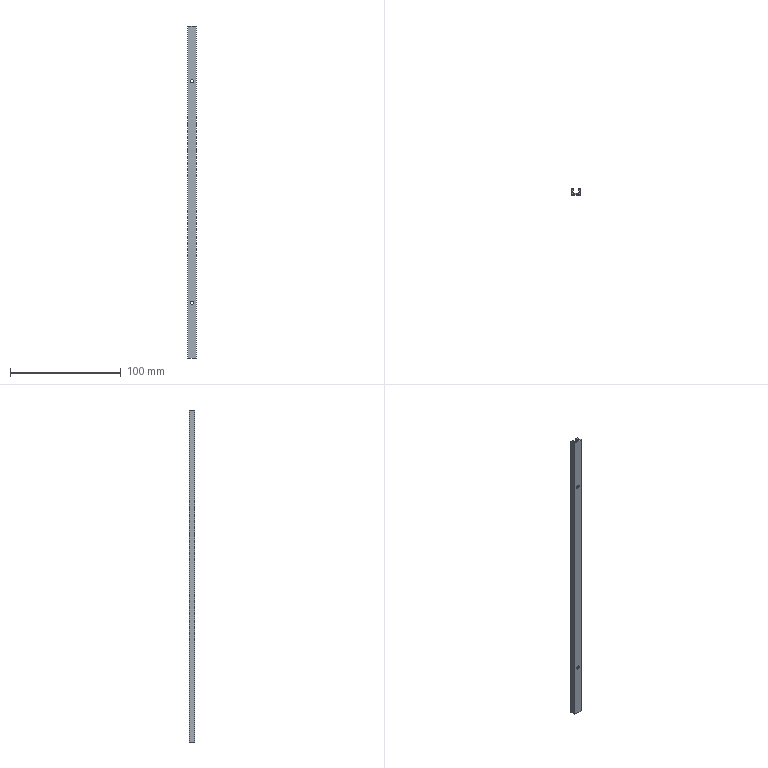Part | SolidWorks | features BaseBody 1 | 1 solid | 22 faces | box 8 x 5 x 300 mm | volume 5669 mm3 | plane 18 | cylinder 4 | commonest cylinder face diameters 3 x4
STEP:
#1=CARTESIAN_POINT('',(0.,0.9,226.5));
#2=VERTEX_POINT('',#1);
#3=CARTESIAN_POINT('',(0.,0.9,223.5));
#4=VERTEX_POINT('',#3);
#5=CARTESIAN_POINT('',(0.,0.9,225.));
#6=DIRECTION('',(0.,-1.,0.));
#7=DIRECTION('',(0.,0.,-1.));
#8=AXIS2_PLACEMENT_3D('',#5,#6,#7);
#9=CIRCLE('',#8,1.5);
#10=EDGE_CURVE('',#2,#4,#9,.T.);
#11=ORIENTED_EDGE('',*,*,#10,.F.);
#12=CARTESIAN_POINT('',(0.,0.,226.5));
#13=VERTEX_POINT('',#12);
#14=CARTESIAN_POINT('',(0.,4.,226.5));
#15=DIRECTION('',(0.,-1.,0.));
#16=VECTOR('',#15,1000.);
#17=LINE('',#14,#16);
#18=EDGE_CURVE('',#2,#13,#17,.T.);
#19=ORIENTED_EDGE('',*,*,#18,.T.);
#20=CARTESIAN_POINT('',(0.,0.,223.5));
#21=VERTEX_POINT('',#20);
#22=CARTESIAN_POINT('',(0.,0.,225.));
#23=DIRECTION('',(0.,1.,0.));
#24=DIRECTION('',(0.,0.,-1.));
#25=AXIS2_PLACEMENT_3D('',#22,#23,#24);
#26=CIRCLE('',#25,1.5);
#27=EDGE_CURVE('',#21,#13,#26,.T.);
#28=ORIENTED_EDGE('',*,*,#27,.F.);
#29=CARTESIAN_POINT('',(0.,4.,223.5));
#30=DIRECTION('',(0.,-1.,0.));
#31=VECTOR('',#30,1000.);
#32=LINE('',#29,#31);
#33=EDGE_CURVE('',#4,#21,#32,.T.);
#34=ORIENTED_EDGE('',*,*,#33,.F.);
#35=EDGE_LOOP('',(#11,#19,#28,#34));
#36=FACE_OUTER_BOUND('',#35,.T.);
#37=CARTESIAN_POINT('',(0.,4.,225.));
#38=DIRECTION('',(0.,-1.,0.));
#39=DIRECTION('',(0.,0.,-1.));
#40=AXIS2_PLACEMENT_3D('',#37,#38,#39);
#41=CYLINDRICAL_SURFACE('',#40,1.5);
#42=ADVANCED_FACE('',(#36),#41,.F.);
#43=CARTESIAN_POINT('',(0.,0.9,26.5));
#44=VERTEX_POINT('',#43);
#45=CARTESIAN_POINT('',(0.,0.9,23.5));
#46=VERTEX_POINT('',#45);
#47=CARTESIAN_POINT('',(0.,0.9,25.));
#48=DIRECTION('',(0.,-1.,0.));
#49=DIRECTION('',(0.,0.,-1.));
#50=AXIS2_PLACEMENT_3D('',#47,#48,#49);
#51=CIRCLE('',#50,1.5);
#52=EDGE_CURVE('',#44,#46,#51,.T.);
#53=ORIENTED_EDGE('',*,*,#52,.F.);
#54=CARTESIAN_POINT('',(0.,0.,26.5));
#55=VERTEX_POINT('',#54);
#56=CARTESIAN_POINT('',(0.,4.,26.5));
#57=DIRECTION('',(0.,-1.,0.));
#58=VECTOR('',#57,1000.);
#59=LINE('',#56,#58);
#60=EDGE_CURVE('',#44,#55,#59,.T.);
#61=ORIENTED_EDGE('',*,*,#60,.T.);
#62=CARTESIAN_POINT('',(0.,0.,23.5));
#63=VERTEX_POINT('',#62);
#64=CARTESIAN_POINT('',(0.,0.,25.));
#65=DIRECTION('',(0.,1.,0.));
#66=DIRECTION('',(0.,0.,-1.));
#67=AXIS2_PLACEMENT_3D('',#64,#65,#66);
#68=CIRCLE('',#67,1.5);
#69=EDGE_CURVE('',#63,#55,#68,.T.);
#70=ORIENTED_EDGE('',*,*,#69,.F.);
#71=CARTESIAN_POINT('',(0.,4.,23.5));
#72=DIRECTION('',(0.,-1.,0.));
#73=VECTOR('',#72,1000.);
#74=LINE('',#71,#73);
#75=EDGE_CURVE('',#46,#63,#74,.T.);
#76=ORIENTED_EDGE('',*,*,#75,.F.);
#77=EDGE_LOOP('',(#53,#61,#70,#76));
#78=FACE_OUTER_BOUND('',#77,.T.);
#79=CARTESIAN_POINT('',(0.,4.,25.));
#80=DIRECTION('',(0.,-1.,0.));
#81=DIRECTION('',(0.,0.,-1.));
#82=AXIS2_PLACEMENT_3D('',#79,#80,#81);
#83=CYLINDRICAL_SURFACE('',#82,1.5);
#84=ADVANCED_FACE('',(#78),#83,.F.);
#85=ORIENTED_EDGE('',*,*,#27,.T.);
#86=CARTESIAN_POINT('',(0.,0.,225.));
#87=DIRECTION('',(0.,1.,0.));
#88=DIRECTION('',(0.,0.,-1.));
#89=AXIS2_PLACEMENT_3D('',#86,#87,#88);
#90=CIRCLE('',#89,1.5);
#91=EDGE_CURVE('',#13,#21,#90,.T.);
#92=ORIENTED_EDGE('',*,*,#91,.T.);
#93=EDGE_LOOP('',(#85,#92));
#94=FACE_BOUND('',#93,.T.);
#95=ORIENTED_EDGE('',*,*,#69,.T.);
#96=CARTESIAN_POINT('',(0.,0.,25.));
#97=DIRECTION('',(0.,1.,0.));
#98=DIRECTION('',(0.,0.,-1.));
#99=AXIS2_PLACEMENT_3D('',#96,#97,#98);
#100=CIRCLE('',#99,1.5);
#101=EDGE_CURVE('',#55,#63,#100,.T.);
#102=ORIENTED_EDGE('',*,*,#101,.T.);
#103=EDGE_LOOP('',(#95,#102));
#104=FACE_BOUND('',#103,.T.);
#105=CARTESIAN_POINT('',(-4.,0.,-25.));
#106=VERTEX_POINT('',#105);
#107=CARTESIAN_POINT('',(4.,0.,-25.));
#108=VERTEX_POINT('',#107);
#109=CARTESIAN_POINT('',(-4.,0.,-25.));
#110=DIRECTION('',(1.,0.,0.));
#111=VECTOR('',#110,1000.);
#112=LINE('',#109,#111);
#113=EDGE_CURVE('',#106,#108,#112,.T.);
#114=ORIENTED_EDGE('',*,*,#113,.T.);
#115=CARTESIAN_POINT('',(4.,0.,275.));
#116=VERTEX_POINT('',#115);
#117=CARTESIAN_POINT('',(4.,0.,0.));
#118=DIRECTION('',(0.,0.,1.));
#119=VECTOR('',#118,1000.);
#120=LINE('',#117,#119);
#121=EDGE_CURVE('',#108,#116,#120,.T.);
#122=ORIENTED_EDGE('',*,*,#121,.T.);
#123=CARTESIAN_POINT('',(-4.,0.,275.));
#124=VERTEX_POINT('',#123);
#125=CARTESIAN_POINT('',(-4.,0.,275.));
#126=DIRECTION('',(-1.,0.,0.));
#127=VECTOR('',#126,1000.);
#128=LINE('',#125,#127);
#129=EDGE_CURVE('',#116,#124,#128,.T.);
#130=ORIENTED_EDGE('',*,*,#129,.T.);
#131=CARTESIAN_POINT('',(-4.,0.,0.));
#132=DIRECTION('',(0.,0.,-1.));
#133=VECTOR('',#132,1000.);
#134=LINE('',#131,#133);
#135=EDGE_CURVE('',#124,#106,#134,.T.);
#136=ORIENTED_EDGE('',*,*,#135,.T.);
#137=EDGE_LOOP('',(#114,#122,#130,#136));
#138=FACE_OUTER_BOUND('',#137,.T.);
#139=CARTESIAN_POINT('',(-4.,0.,0.));
#140=DIRECTION('',(0.,-1.,0.));
#141=DIRECTION('',(0.,0.,-1.));
#142=AXIS2_PLACEMENT_3D('',#139,#140,#141);
#143=PLANE('',#142);
#144=ADVANCED_FACE('',(#94,#104,#138),#143,.T.);
#145=ORIENTED_EDGE('',*,*,#18,.F.);
#146=CARTESIAN_POINT('',(0.,0.9,225.));
#147=DIRECTION('',(0.,-1.,0.));
#148=DIRECTION('',(0.,0.,-1.));
#149=AXIS2_PLACEMENT_3D('',#146,#147,#148);
#150=CIRCLE('',#149,1.5);
#151=EDGE_CURVE('',#4,#2,#150,.T.);
#152=ORIENTED_EDGE('',*,*,#151,.F.);
#153=ORIENTED_EDGE('',*,*,#33,.T.);
#154=ORIENTED_EDGE('',*,*,#91,.F.);
#155=EDGE_LOOP('',(#145,#152,#153,#154));
#156=FACE_OUTER_BOUND('',#155,.T.);
#157=CARTESIAN_POINT('',(0.,4.,225.));
#158=DIRECTION('',(0.,-1.,0.));
#159=DIRECTION('',(0.,0.,-1.));
#160=AXIS2_PLACEMENT_3D('',#157,#158,#159);
#161=CYLINDRICAL_SURFACE('',#160,1.5);
#162=ADVANCED_FACE('',(#156),#161,.F.);
#163=ORIENTED_EDGE('',*,*,#60,.F.);
#164=CARTESIAN_POINT('',(0.,0.9,25.));
#165=DIRECTION('',(0.,-1.,0.));
#166=DIRECTION('',(0.,0.,-1.));
#167=AXIS2_PLACEMENT_3D('',#164,#165,#166);
#168=CIRCLE('',#167,1.5);
#169=EDGE_CURVE('',#46,#44,#168,.T.);
#170=ORIENTED_EDGE('',*,*,#169,.F.);
#171=ORIENTED_EDGE('',*,*,#75,.T.);
#172=ORIENTED_EDGE('',*,*,#101,.F.);
#173=EDGE_LOOP('',(#163,#170,#171,#172));
#174=FACE_OUTER_BOUND('',#173,.T.);
#175=CARTESIAN_POINT('',(0.,4.,25.));
#176=DIRECTION('',(0.,-1.,0.));
#177=DIRECTION('',(0.,0.,-1.));
#178=AXIS2_PLACEMENT_3D('',#175,#176,#177);
#179=CYLINDRICAL_SURFACE('',#178,1.5);
#180=ADVANCED_FACE('',(#174),#179,.F.);
#181=CARTESIAN_POINT('',(4.,5.,275.));
#182=VERTEX_POINT('',#181);
#183=CARTESIAN_POINT('',(4.,0.,275.));
#184=DIRECTION('',(0.,-1.,0.));
#185=VECTOR('',#184,1000.);
#186=LINE('',#183,#185);
#187=EDGE_CURVE('',#182,#116,#186,.T.);
#188=ORIENTED_EDGE('',*,*,#187,.T.);
#189=ORIENTED_EDGE('',*,*,#121,.F.);
#190=CARTESIAN_POINT('',(4.,5.,-25.));
#191=VERTEX_POINT('',#190);
#192=CARTESIAN_POINT('',(4.,0.,-25.));
#193=DIRECTION('',(0.,1.,0.));
#194=VECTOR('',#193,1000.);
#195=LINE('',#192,#194);
#196=EDGE_CURVE('',#108,#191,#195,.T.);
#197=ORIENTED_EDGE('',*,*,#196,.T.);
#198=CARTESIAN_POINT('',(4.,5.,0.));
#199=DIRECTION('',(0.,0.,1.));
#200=VECTOR('',#199,1000.);
#201=LINE('',#198,#200);
#202=EDGE_CURVE('',#191,#182,#201,.T.);
#203=ORIENTED_EDGE('',*,*,#202,.T.);
#204=EDGE_LOOP('',(#188,#189,#197,#203));
#205=FACE_OUTER_BOUND('',#204,.T.);
#206=CARTESIAN_POINT('',(4.,0.,0.));
#207=DIRECTION('',(1.,0.,0.));
#208=DIRECTION('',(0.,0.,-1.));
#209=AXIS2_PLACEMENT_3D('',#206,#207,#208);
#210=PLANE('',#209);
#211=ADVANCED_FACE('',(#205),#210,.T.);
#212=ORIENTED_EDGE('',*,*,#113,.F.);
#213=CARTESIAN_POINT('',(-4.,5.,-25.));
#214=VERTEX_POINT('',#213);
#215=CARTESIAN_POINT('',(-4.,0.,-25.));
#216=DIRECTION('',(0.,-1.,0.));
#217=VECTOR('',#216,1000.);
#218=LINE('',#215,#217);
#219=EDGE_CURVE('',#214,#106,#218,.T.);
#220=ORIENTED_EDGE('',*,*,#219,.F.);
#221=CARTESIAN_POINT('',(-2.1,5.,-25.));
#222=VERTEX_POINT('',#221);
#223=CARTESIAN_POINT('',(0.,5.,-25.));
#224=DIRECTION('',(-1.,0.,0.));
#225=VECTOR('',#224,1000.);
#226=LINE('',#223,#225);
#227=EDGE_CURVE('',#222,#214,#226,.T.);
#228=ORIENTED_EDGE('',*,*,#227,.F.);
#229=CARTESIAN_POINT('',(-2.1,4.2,-25.));
#230=VERTEX_POINT('',#229);
#231=CARTESIAN_POINT('',(-2.1,4.2,-25.));
#232=DIRECTION('',(0.,1.,0.));
#233=VECTOR('',#232,1000.);
#234=LINE('',#231,#233);
#235=EDGE_CURVE('',#230,#222,#234,.T.);
#236=ORIENTED_EDGE('',*,*,#235,.F.);
#237=CARTESIAN_POINT('',(-2.9,4.2,-25.));
#238=VERTEX_POINT('',#237);
#239=CARTESIAN_POINT('',(-2.9,4.2,-25.));
#240=DIRECTION('',(1.,0.,0.));
#241=VECTOR('',#240,1000.);
#242=LINE('',#239,#241);
#243=EDGE_CURVE('',#238,#230,#242,.T.);
#244=ORIENTED_EDGE('',*,*,#243,.F.);
#245=CARTESIAN_POINT('',(-2.9,1.8,-25.));
#246=VERTEX_POINT('',#245);
#247=CARTESIAN_POINT('',(-2.9,0.,-25.));
#248=DIRECTION('',(0.,1.,0.));
#249=VECTOR('',#248,1000.);
#250=LINE('',#247,#249);
#251=EDGE_CURVE('',#246,#238,#250,.T.);
#252=ORIENTED_EDGE('',*,*,#251,.F.);
#253=CARTESIAN_POINT('',(-2.1,1.8,-25.));
#254=VERTEX_POINT('',#253);
#255=CARTESIAN_POINT('',(-2.1,1.8,-25.));
#256=DIRECTION('',(-1.,0.,0.));
#257=VECTOR('',#256,1000.);
#258=LINE('',#255,#257);
#259=EDGE_CURVE('',#254,#246,#258,.T.);
#260=ORIENTED_EDGE('',*,*,#259,.F.);
#261=CARTESIAN_POINT('',(-2.1,0.9,-25.));
#262=VERTEX_POINT('',#261);
#263=CARTESIAN_POINT('',(-2.1,0.9,-25.));
#264=DIRECTION('',(0.,1.,0.));
#265=VECTOR('',#264,1000.);
#266=LINE('',#263,#265);
#267=EDGE_CURVE('',#262,#254,#266,.T.);
#268=ORIENTED_EDGE('',*,*,#267,.F.);
#269=CARTESIAN_POINT('',(2.1,0.9,-25.));
#270=VERTEX_POINT('',#269);
#271=CARTESIAN_POINT('',(0.,0.9,-25.));
#272=DIRECTION('',(-1.,0.,0.));
#273=VECTOR('',#272,1000.);
#274=LINE('',#271,#273);
#275=EDGE_CURVE('',#270,#262,#274,.T.);
#276=ORIENTED_EDGE('',*,*,#275,.F.);
#277=CARTESIAN_POINT('',(2.1,1.8,-25.));
#278=VERTEX_POINT('',#277);
#279=CARTESIAN_POINT('',(2.1,1.8,-25.));
#280=DIRECTION('',(0.,-1.,0.));
#281=VECTOR('',#280,1000.);
#282=LINE('',#279,#281);
#283=EDGE_CURVE('',#278,#270,#282,.T.);
#284=ORIENTED_EDGE('',*,*,#283,.F.);
#285=CARTESIAN_POINT('',(2.9,1.8,-25.));
#286=VERTEX_POINT('',#285);
#287=CARTESIAN_POINT('',(2.9,1.8,-25.));
#288=DIRECTION('',(-1.,0.,0.));
#289=VECTOR('',#288,1000.);
#290=LINE('',#287,#289);
#291=EDGE_CURVE('',#286,#278,#290,.T.);
#292=ORIENTED_EDGE('',*,*,#291,.F.);
#293=CARTESIAN_POINT('',(2.9,4.2,-25.));
#294=VERTEX_POINT('',#293);
#295=CARTESIAN_POINT('',(2.9,0.,-25.));
#296=DIRECTION('',(0.,-1.,0.));
#297=VECTOR('',#296,1000.);
#298=LINE('',#295,#297);
#299=EDGE_CURVE('',#294,#286,#298,.T.);
#300=ORIENTED_EDGE('',*,*,#299,.F.);
#301=CARTESIAN_POINT('',(2.1,4.2,-25.));
#302=VERTEX_POINT('',#301);
#303=CARTESIAN_POINT('',(2.1,4.2,-25.));
#304=DIRECTION('',(1.,0.,0.));
#305=VECTOR('',#304,1000.);
#306=LINE('',#303,#305);
#307=EDGE_CURVE('',#302,#294,#306,.T.);
#308=ORIENTED_EDGE('',*,*,#307,.F.);
#309=CARTESIAN_POINT('',(2.1,5.,-25.));
#310=VERTEX_POINT('',#309);
#311=CARTESIAN_POINT('',(2.1,5.,-25.));
#312=DIRECTION('',(0.,-1.,0.));
#313=VECTOR('',#312,1000.);
#314=LINE('',#311,#313);
#315=EDGE_CURVE('',#310,#302,#314,.T.);
#316=ORIENTED_EDGE('',*,*,#315,.F.);
#317=CARTESIAN_POINT('',(0.,5.,-25.));
#318=DIRECTION('',(-1.,0.,0.));
#319=VECTOR('',#318,1000.);
#320=LINE('',#317,#319);
#321=EDGE_CURVE('',#191,#310,#320,.T.);
#322=ORIENTED_EDGE('',*,*,#321,.F.);
#323=ORIENTED_EDGE('',*,*,#196,.F.);
#324=EDGE_LOOP('',(#212,#220,#228,#236,#244,#252,#260,#268,#276,#284,#292,#300,#308,#316,#322,#323));
#325=FACE_OUTER_BOUND('',#324,.T.);
#326=CARTESIAN_POINT('',(0.,0.,-25.));
#327=DIRECTION('',(0.,0.,1.));
#328=DIRECTION('',(1.,0.,0.));
#329=AXIS2_PLACEMENT_3D('',#326,#327,#328);
#330=PLANE('',#329);
#331=ADVANCED_FACE('',(#325),#330,.F.);
#332=CARTESIAN_POINT('',(-4.,5.,275.));
#333=VERTEX_POINT('',#332);
#334=CARTESIAN_POINT('',(-4.,5.,275.));
#335=DIRECTION('',(0.,1.,0.));
#336=VECTOR('',#335,1000.);
#337=LINE('',#334,#336);
#338=EDGE_CURVE('',#124,#333,#337,.T.);
#339=ORIENTED_EDGE('',*,*,#338,.T.);
#340=CARTESIAN_POINT('',(-4.,5.,0.));
#341=DIRECTION('',(0.,0.,-1.));
#342=VECTOR('',#341,1000.);
#343=LINE('',#340,#342);
#344=EDGE_CURVE('',#333,#214,#343,.T.);
#345=ORIENTED_EDGE('',*,*,#344,.T.);
#346=ORIENTED_EDGE('',*,*,#219,.T.);
#347=ORIENTED_EDGE('',*,*,#135,.F.);
#348=EDGE_LOOP('',(#339,#345,#346,#347));
#349=FACE_OUTER_BOUND('',#348,.T.);
#350=CARTESIAN_POINT('',(-4.,5.,0.));
#351=DIRECTION('',(-1.,0.,0.));
#352=DIRECTION('',(0.,0.,1.));
#353=AXIS2_PLACEMENT_3D('',#350,#351,#352);
#354=PLANE('',#353);
#355=ADVANCED_FACE('',(#349),#354,.T.);
#356=CARTESIAN_POINT('',(2.1,1.8,275.));
#357=VERTEX_POINT('',#356);
#358=CARTESIAN_POINT('',(2.9,1.8,275.));
#359=VERTEX_POINT('',#358);
#360=CARTESIAN_POINT('',(2.9,1.8,275.));
#361=DIRECTION('',(1.,0.,0.));
#362=VECTOR('',#361,1000.);
#363=LINE('',#360,#362);
#364=EDGE_CURVE('',#357,#359,#363,.T.);
#365=ORIENTED_EDGE('',*,*,#364,.F.);
#366=CARTESIAN_POINT('',(2.1,0.9,275.));
#367=VERTEX_POINT('',#366);
#368=CARTESIAN_POINT('',(2.1,1.8,275.));
#369=DIRECTION('',(0.,1.,0.));
#370=VECTOR('',#369,1000.);
#371=LINE('',#368,#370);
#372=EDGE_CURVE('',#367,#357,#371,.T.);
#373=ORIENTED_EDGE('',*,*,#372,.F.);
#374=CARTESIAN_POINT('',(-2.1,0.9,275.));
#375=VERTEX_POINT('',#374);
#376=CARTESIAN_POINT('',(0.,0.9,275.));
#377=DIRECTION('',(-1.,0.,0.));
#378=VECTOR('',#377,1000.);
#379=LINE('',#376,#378);
#380=EDGE_CURVE('',#367,#375,#379,.T.);
#381=ORIENTED_EDGE('',*,*,#380,.T.);
#382=CARTESIAN_POINT('',(-2.1,1.8,275.));
#383=VERTEX_POINT('',#382);
#384=CARTESIAN_POINT('',(-2.1,0.9,275.));
#385=DIRECTION('',(0.,-1.,0.));
#386=VECTOR('',#385,1000.);
#387=LINE('',#384,#386);
#388=EDGE_CURVE('',#383,#375,#387,.T.);
#389=ORIENTED_EDGE('',*,*,#388,.F.);
#390=CARTESIAN_POINT('',(-2.9,1.8,275.));
#391=VERTEX_POINT('',#390);
#392=CARTESIAN_POINT('',(-2.1,1.8,275.));
#393=DIRECTION('',(1.,0.,0.));
#394=VECTOR('',#393,1000.);
#395=LINE('',#392,#394);
#396=EDGE_CURVE('',#391,#383,#395,.T.);
#397=ORIENTED_EDGE('',*,*,#396,.F.);
#398=CARTESIAN_POINT('',(-2.9,4.2,275.));
#399=VERTEX_POINT('',#398);
#400=CARTESIAN_POINT('',(-2.9,0.,275.));
#401=DIRECTION('',(0.,1.,0.));
#402=VECTOR('',#401,1000.);
#403=LINE('',#400,#402);
#404=EDGE_CURVE('',#391,#399,#403,.T.);
#405=ORIENTED_EDGE('',*,*,#404,.T.);
#406=CARTESIAN_POINT('',(-2.1,4.2,275.));
#407=VERTEX_POINT('',#406);
#408=CARTESIAN_POINT('',(-2.9,4.2,275.));
#409=DIRECTION('',(-1.,0.,0.));
#410=VECTOR('',#409,1000.);
#411=LINE('',#408,#410);
#412=EDGE_CURVE('',#407,#399,#411,.T.);
#413=ORIENTED_EDGE('',*,*,#412,.F.);
#414=CARTESIAN_POINT('',(-2.1,5.,275.));
#415=VERTEX_POINT('',#414);
#416=CARTESIAN_POINT('',(-2.1,4.2,275.));
#417=DIRECTION('',(0.,-1.,0.));
#418=VECTOR('',#417,1000.);
#419=LINE('',#416,#418);
#420=EDGE_CURVE('',#415,#407,#419,.T.);
#421=ORIENTED_EDGE('',*,*,#420,.F.);
#422=CARTESIAN_POINT('',(0.,5.,275.));
#423=DIRECTION('',(-1.,0.,0.));
#424=VECTOR('',#423,1000.);
#425=LINE('',#422,#424);
#426=EDGE_CURVE('',#415,#333,#425,.T.);
#427=ORIENTED_EDGE('',*,*,#426,.T.);
#428=ORIENTED_EDGE('',*,*,#338,.F.);
#429=ORIENTED_EDGE('',*,*,#129,.F.);
#430=ORIENTED_EDGE('',*,*,#187,.F.);
#431=CARTESIAN_POINT('',(2.1,5.,275.));
#432=VERTEX_POINT('',#431);
#433=CARTESIAN_POINT('',(0.,5.,275.));
#434=DIRECTION('',(-1.,0.,0.));
#435=VECTOR('',#434,1000.);
#436=LINE('',#433,#435);
#437=EDGE_CURVE('',#182,#432,#436,.T.);
#438=ORIENTED_EDGE('',*,*,#437,.T.);
#439=CARTESIAN_POINT('',(2.1,4.2,275.));
#440=VERTEX_POINT('',#439);
#441=CARTESIAN_POINT('',(2.1,5.,275.));
#442=DIRECTION('',(0.,1.,0.));
#443=VECTOR('',#442,1000.);
#444=LINE('',#441,#443);
#445=EDGE_CURVE('',#440,#432,#444,.T.);
#446=ORIENTED_EDGE('',*,*,#445,.F.);
#447=CARTESIAN_POINT('',(2.9,4.2,275.));
#448=VERTEX_POINT('',#447);
#449=CARTESIAN_POINT('',(2.1,4.2,275.));
#450=DIRECTION('',(-1.,0.,0.));
#451=VECTOR('',#450,1000.);
#452=LINE('',#449,#451);
#453=EDGE_CURVE('',#448,#440,#452,.T.);
#454=ORIENTED_EDGE('',*,*,#453,.F.);
#455=CARTESIAN_POINT('',(2.9,0.,275.));
#456=DIRECTION('',(0.,-1.,0.));
#457=VECTOR('',#456,1000.);
#458=LINE('',#455,#457);
#459=EDGE_CURVE('',#448,#359,#458,.T.);
#460=ORIENTED_EDGE('',*,*,#459,.T.);
#461=EDGE_LOOP('',(#365,#373,#381,#389,#397,#405,#413,#421,#427,#428,#429,#430,#438,#446,#454,#460));
#462=FACE_OUTER_BOUND('',#461,.T.);
#463=CARTESIAN_POINT('',(0.,0.,275.));
#464=DIRECTION('',(0.,0.,1.));
#465=DIRECTION('',(1.,0.,0.));
#466=AXIS2_PLACEMENT_3D('',#463,#464,#465);
#467=PLANE('',#466);
#468=ADVANCED_FACE('',(#462),#467,.T.);
#469=ORIENTED_EDGE('',*,*,#151,.T.);
#470=ORIENTED_EDGE('',*,*,#10,.T.);
#471=EDGE_LOOP('',(#469,#470));
#472=FACE_BOUND('',#471,.T.);
#473=ORIENTED_EDGE('',*,*,#169,.T.);
#474=ORIENTED_EDGE('',*,*,#52,.T.);
#475=EDGE_LOOP('',(#473,#474));
#476=FACE_BOUND('',#475,.T.);
#477=ORIENTED_EDGE('',*,*,#275,.T.);
#478=CARTESIAN_POINT('',(-2.1,0.9,0.));
#479=DIRECTION('',(0.,0.,1.));
#480=VECTOR('',#479,1000.);
#481=LINE('',#478,#480);
#482=EDGE_CURVE('',#262,#375,#481,.T.);
#483=ORIENTED_EDGE('',*,*,#482,.T.);
#484=ORIENTED_EDGE('',*,*,#380,.F.);
#485=CARTESIAN_POINT('',(2.1,0.9,0.));
#486=DIRECTION('',(0.,0.,-1.));
#487=VECTOR('',#486,1000.);
#488=LINE('',#485,#487);
#489=EDGE_CURVE('',#367,#270,#488,.T.);
#490=ORIENTED_EDGE('',*,*,#489,.T.);
#491=EDGE_LOOP('',(#477,#483,#484,#490));
#492=FACE_OUTER_BOUND('',#491,.T.);
#493=CARTESIAN_POINT('',(2.1,0.9,0.));
#494=DIRECTION('',(0.,1.,0.));
#495=DIRECTION('',(0.,0.,1.));
#496=AXIS2_PLACEMENT_3D('',#493,#494,#495);
#497=PLANE('',#496);
#498=ADVANCED_FACE('',(#472,#476,#492),#497,.T.);
#499=ORIENTED_EDGE('',*,*,#437,.F.);
#500=ORIENTED_EDGE('',*,*,#202,.F.);
#501=ORIENTED_EDGE('',*,*,#321,.T.);
#502=CARTESIAN_POINT('',(2.1,5.,0.));
#503=DIRECTION('',(0.,0.,1.));
#504=VECTOR('',#503,1000.);
#505=LINE('',#502,#504);
#506=EDGE_CURVE('',#310,#432,#505,.T.);
#507=ORIENTED_EDGE('',*,*,#506,.T.);
#508=EDGE_LOOP('',(#499,#500,#501,#507));
#509=FACE_OUTER_BOUND('',#508,.T.);
#510=CARTESIAN_POINT('',(4.,5.,0.));
#511=DIRECTION('',(0.,1.,0.));
#512=DIRECTION('',(0.,0.,1.));
#513=AXIS2_PLACEMENT_3D('',#510,#511,#512);
#514=PLANE('',#513);
#515=ADVANCED_FACE('',(#509),#514,.T.);
#516=ORIENTED_EDGE('',*,*,#426,.F.);
#517=CARTESIAN_POINT('',(-2.1,5.,0.));
#518=DIRECTION('',(0.,0.,-1.));
#519=VECTOR('',#518,1000.);
#520=LINE('',#517,#519);
#521=EDGE_CURVE('',#415,#222,#520,.T.);
#522=ORIENTED_EDGE('',*,*,#521,.T.);
#523=ORIENTED_EDGE('',*,*,#227,.T.);
#524=ORIENTED_EDGE('',*,*,#344,.F.);
#525=EDGE_LOOP('',(#516,#522,#523,#524));
#526=FACE_OUTER_BOUND('',#525,.T.);
#527=CARTESIAN_POINT('',(-2.1,5.,0.));
#528=DIRECTION('',(0.,1.,0.));
#529=DIRECTION('',(0.,0.,1.));
#530=AXIS2_PLACEMENT_3D('',#527,#528,#529);
#531=PLANE('',#530);
#532=ADVANCED_FACE('',(#526),#531,.T.);
#533=ORIENTED_EDGE('',*,*,#404,.F.);
#534=CARTESIAN_POINT('',(-2.9,1.8,0.));
#535=DIRECTION('',(0.,0.,-1.));
#536=VECTOR('',#535,1000.);
#537=LINE('',#534,#536);
#538=EDGE_CURVE('',#391,#246,#537,.T.);
#539=ORIENTED_EDGE('',*,*,#538,.T.);
#540=ORIENTED_EDGE('',*,*,#251,.T.);
#541=CARTESIAN_POINT('',(-2.9,4.2,0.));
#542=DIRECTION('',(0.,0.,1.));
#543=VECTOR('',#542,1000.);
#544=LINE('',#541,#543);
#545=EDGE_CURVE('',#238,#399,#544,.T.);
#546=ORIENTED_EDGE('',*,*,#545,.T.);
#547=EDGE_LOOP('',(#533,#539,#540,#546));
#548=FACE_OUTER_BOUND('',#547,.T.);
#549=CARTESIAN_POINT('',(-2.9,1.8,0.));
#550=DIRECTION('',(1.,0.,0.));
#551=DIRECTION('',(0.,0.,-1.));
#552=AXIS2_PLACEMENT_3D('',#549,#550,#551);
#553=PLANE('',#552);
#554=ADVANCED_FACE('',(#548),#553,.T.);
#555=ORIENTED_EDGE('',*,*,#459,.F.);
#556=CARTESIAN_POINT('',(2.9,4.2,0.));
#557=DIRECTION('',(0.,0.,-1.));
#558=VECTOR('',#557,1000.);
#559=LINE('',#556,#558);
#560=EDGE_CURVE('',#448,#294,#559,.T.);
#561=ORIENTED_EDGE('',*,*,#560,.T.);
#562=ORIENTED_EDGE('',*,*,#299,.T.);
#563=CARTESIAN_POINT('',(2.9,1.8,0.));
#564=DIRECTION('',(0.,0.,1.));
#565=VECTOR('',#564,1000.);
#566=LINE('',#563,#565);
#567=EDGE_CURVE('',#286,#359,#566,.T.);
#568=ORIENTED_EDGE('',*,*,#567,.T.);
#569=EDGE_LOOP('',(#555,#561,#562,#568));
#570=FACE_OUTER_BOUND('',#569,.T.);
#571=CARTESIAN_POINT('',(2.9,4.2,0.));
#572=DIRECTION('',(-1.,0.,0.));
#573=DIRECTION('',(0.,0.,1.));
#574=AXIS2_PLACEMENT_3D('',#571,#572,#573);
#575=PLANE('',#574);
#576=ADVANCED_FACE('',(#570),#575,.T.);
#577=ORIENTED_EDGE('',*,*,#388,.T.);
#578=ORIENTED_EDGE('',*,*,#482,.F.);
#579=ORIENTED_EDGE('',*,*,#267,.T.);
#580=CARTESIAN_POINT('',(-2.1,1.8,0.));
#581=DIRECTION('',(0.,0.,1.));
#582=VECTOR('',#581,1000.);
#583=LINE('',#580,#582);
#584=EDGE_CURVE('',#254,#383,#583,.T.);
#585=ORIENTED_EDGE('',*,*,#584,.T.);
#586=EDGE_LOOP('',(#577,#578,#579,#585));
#587=FACE_OUTER_BOUND('',#586,.T.);
#588=CARTESIAN_POINT('',(-2.1,0.9,0.));
#589=DIRECTION('',(1.,0.,0.));
#590=DIRECTION('',(0.,0.,-1.));
#591=AXIS2_PLACEMENT_3D('',#588,#589,#590);
#592=PLANE('',#591);
#593=ADVANCED_FACE('',(#587),#592,.T.);
#594=ORIENTED_EDGE('',*,*,#372,.T.);
#595=CARTESIAN_POINT('',(2.1,1.8,0.));
#596=DIRECTION('',(0.,0.,-1.));
#597=VECTOR('',#596,1000.);
#598=LINE('',#595,#597);
#599=EDGE_CURVE('',#357,#278,#598,.T.);
#600=ORIENTED_EDGE('',*,*,#599,.T.);
#601=ORIENTED_EDGE('',*,*,#283,.T.);
#602=ORIENTED_EDGE('',*,*,#489,.F.);
#603=EDGE_LOOP('',(#594,#600,#601,#602));
#604=FACE_OUTER_BOUND('',#603,.T.);
#605=CARTESIAN_POINT('',(2.1,1.8,0.));
#606=DIRECTION('',(-1.,0.,0.));
#607=DIRECTION('',(0.,0.,1.));
#608=AXIS2_PLACEMENT_3D('',#605,#606,#607);
#609=PLANE('',#608);
#610=ADVANCED_FACE('',(#604),#609,.T.);
#611=ORIENTED_EDGE('',*,*,#445,.T.);
#612=ORIENTED_EDGE('',*,*,#506,.F.);
#613=ORIENTED_EDGE('',*,*,#315,.T.);
#614=CARTESIAN_POINT('',(2.1,4.2,0.));
#615=DIRECTION('',(0.,0.,1.));
#616=VECTOR('',#615,1000.);
#617=LINE('',#614,#616);
#618=EDGE_CURVE('',#302,#440,#617,.T.);
#619=ORIENTED_EDGE('',*,*,#618,.T.);
#620=EDGE_LOOP('',(#611,#612,#613,#619));
#621=FACE_OUTER_BOUND('',#620,.T.);
#622=CARTESIAN_POINT('',(2.1,5.,0.));
#623=DIRECTION('',(-1.,0.,0.));
#624=DIRECTION('',(0.,0.,1.));
#625=AXIS2_PLACEMENT_3D('',#622,#623,#624);
#626=PLANE('',#625);
#627=ADVANCED_FACE('',(#621),#626,.T.);
#628=ORIENTED_EDGE('',*,*,#420,.T.);
#629=CARTESIAN_POINT('',(-2.1,4.2,0.));
#630=DIRECTION('',(0.,0.,-1.));
#631=VECTOR('',#630,1000.);
#632=LINE('',#629,#631);
#633=EDGE_CURVE('',#407,#230,#632,.T.);
#634=ORIENTED_EDGE('',*,*,#633,.T.);
#635=ORIENTED_EDGE('',*,*,#235,.T.);
#636=ORIENTED_EDGE('',*,*,#521,.F.);
#637=EDGE_LOOP('',(#628,#634,#635,#636));
#638=FACE_OUTER_BOUND('',#637,.T.);
#639=CARTESIAN_POINT('',(-2.1,4.2,0.));
#640=DIRECTION('',(1.,0.,0.));
#641=DIRECTION('',(0.,0.,-1.));
#642=AXIS2_PLACEMENT_3D('',#639,#640,#641);
#643=PLANE('',#642);
#644=ADVANCED_FACE('',(#638),#643,.T.);
#645=ORIENTED_EDGE('',*,*,#396,.T.);
#646=ORIENTED_EDGE('',*,*,#584,.F.);
#647=ORIENTED_EDGE('',*,*,#259,.T.);
#648=ORIENTED_EDGE('',*,*,#538,.F.);
#649=EDGE_LOOP('',(#645,#646,#647,#648));
#650=FACE_OUTER_BOUND('',#649,.T.);
#651=CARTESIAN_POINT('',(-2.1,1.8,0.));
#652=DIRECTION('',(0.,1.,0.));
#653=DIRECTION('',(0.,0.,1.));
#654=AXIS2_PLACEMENT_3D('',#651,#652,#653);
#655=PLANE('',#654);
#656=ADVANCED_FACE('',(#650),#655,.T.);
#657=ORIENTED_EDGE('',*,*,#412,.T.);
#658=ORIENTED_EDGE('',*,*,#545,.F.);
#659=ORIENTED_EDGE('',*,*,#243,.T.);
#660=ORIENTED_EDGE('',*,*,#633,.F.);
#661=EDGE_LOOP('',(#657,#658,#659,#660));
#662=FACE_OUTER_BOUND('',#661,.T.);
#663=CARTESIAN_POINT('',(-2.9,4.2,0.));
#664=DIRECTION('',(0.,-1.,0.));
#665=DIRECTION('',(0.,0.,-1.));
#666=AXIS2_PLACEMENT_3D('',#663,#664,#665);
#667=PLANE('',#666);
#668=ADVANCED_FACE('',(#662),#667,.T.);
#669=ORIENTED_EDGE('',*,*,#453,.T.);
#670=ORIENTED_EDGE('',*,*,#618,.F.);
#671=ORIENTED_EDGE('',*,*,#307,.T.);
#672=ORIENTED_EDGE('',*,*,#560,.F.);
#673=EDGE_LOOP('',(#669,#670,#671,#672));
#674=FACE_OUTER_BOUND('',#673,.T.);
#675=CARTESIAN_POINT('',(2.1,4.2,0.));
#676=DIRECTION('',(0.,-1.,0.));
#677=DIRECTION('',(0.,0.,-1.));
#678=AXIS2_PLACEMENT_3D('',#675,#676,#677);
#679=PLANE('',#678);
#680=ADVANCED_FACE('',(#674),#679,.T.);
#681=ORIENTED_EDGE('',*,*,#364,.T.);
#682=ORIENTED_EDGE('',*,*,#567,.F.);
#683=ORIENTED_EDGE('',*,*,#291,.T.);
#684=ORIENTED_EDGE('',*,*,#599,.F.);
#685=EDGE_LOOP('',(#681,#682,#683,#684));
#686=FACE_OUTER_BOUND('',#685,.T.);
#687=CARTESIAN_POINT('',(2.9,1.8,0.));
#688=DIRECTION('',(0.,1.,0.));
#689=DIRECTION('',(0.,0.,1.));
#690=AXIS2_PLACEMENT_3D('',#687,#688,#689);
#691=PLANE('',#690);
#692=ADVANCED_FACE('',(#686),#691,.T.);
#693=CLOSED_SHELL('',(#42,#84,#144,#162,#180,#211,#331,#355,#468,#498,#515,#532,#554,#576,#593,#610,#627,#644,#656,#668,#680,#692));
#694=MANIFOLD_SOLID_BREP('',#693);
#695=CARTESIAN_POINT('',(0.,0.,0.));
#696=DIRECTION('',(0.,0.,1.));
#697=DIRECTION('',(1.,0.,0.));
#698=AXIS2_PLACEMENT_3D('',#695,#696,#697);
#699=(LENGTH_UNIT()NAMED_UNIT(*)SI_UNIT(.MILLI.,.METRE.));
#700=UNCERTAINTY_MEASURE_WITH_UNIT(LENGTH_MEASURE(0.00001),#699,'','');
#701=(NAMED_UNIT(*)PLANE_ANGLE_UNIT()SI_UNIT($,.RADIAN.));
#702=(NAMED_UNIT(*)SI_UNIT($,.STERADIAN.)SOLID_ANGLE_UNIT());
#703=(GEOMETRIC_REPRESENTATION_CONTEXT(3)GLOBAL_UNCERTAINTY_ASSIGNED_CONTEXT((#700))GLOBAL_UNIT_ASSIGNED_CONTEXT((#699,#701,#702))REPRESENTATION_CONTEXT('',''));
#704=ADVANCED_BREP_SHAPE_REPRESENTATION('',(#694,#698),#703);